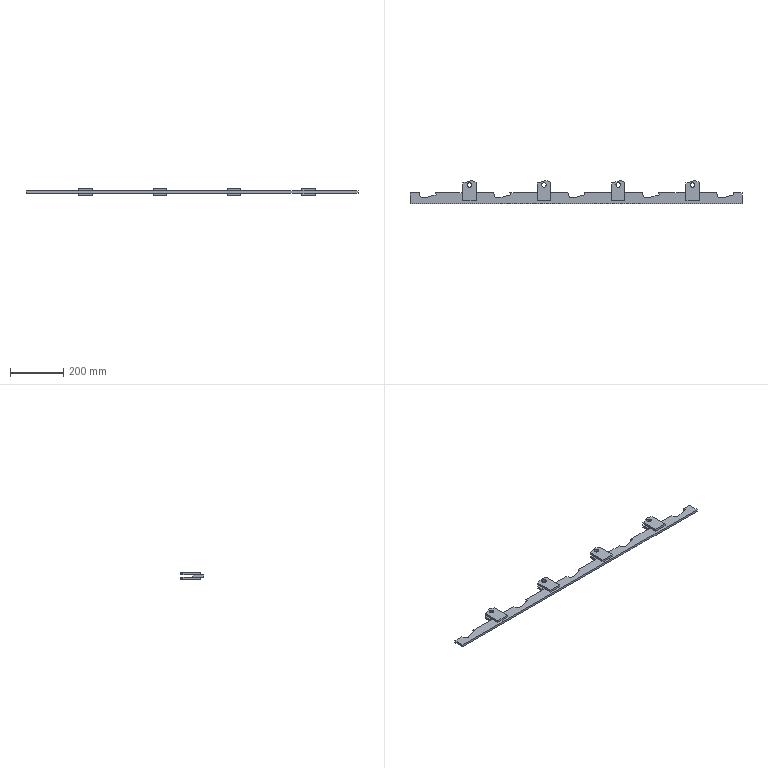Part | STEP file | Connecting plate assembly 3_Default<As machined> | 9 solids | 103 faces | box 1250 x 86.845 x 24 mm | volume 582349 mm3 | plane 82 | cylinder 21 | commonest cylinder face diameters 17 x16 30 x5